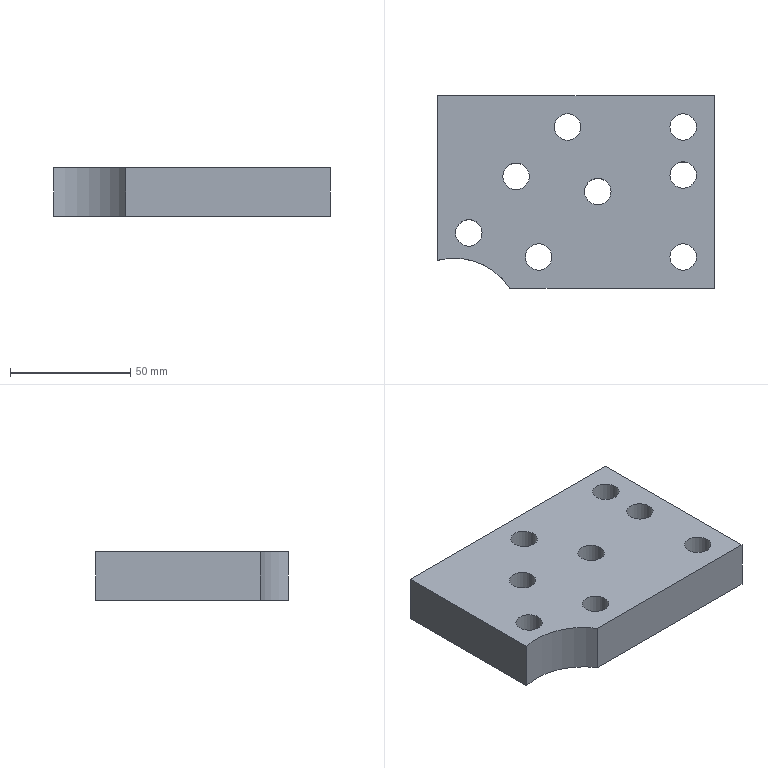Part | STEP file | 117_id2854_x_t | 1 solid | 15 faces | box 115 x 80 x 20 mm | volume 163028 mm3 | cylinder 9 | plane 6 | commonest cylinder face diameters 11 x8 55 x1
STEP:
#1=CARTESIAN_POINT('',(0.,0.,0.));
#2=DIRECTION('',(0.,0.,1.));
#3=DIRECTION('',(1.,0.,0.));
#4=AXIS2_PLACEMENT_3D('',#1,#2,#3);
#5=CARTESIAN_POINT('',(1208.57,-125.851,105.));
#6=VERTEX_POINT('',#5);
#7=CARTESIAN_POINT('',(1203.07,-125.851,105.));
#8=DIRECTION('',(0.,0.,-1.));
#9=DIRECTION('',(1.,0.,0.));
#10=AXIS2_PLACEMENT_3D('',#7,#8,#9);
#11=CIRCLE('',#10,5.5);
#12=CARTESIAN_POINT('',(1128.,-115.,105.));
#13=DIRECTION('',(0.,0.,1.));
#14=DIRECTION('',(-1.,0.,0.));
#15=AXIS2_PLACEMENT_3D('',#12,#13,#14);
#16=PLANE('',#15);
#17=CARTESIAN_POINT('',(-80.57,10.851));
#18=CARTESIAN_POINT('',(-80.57,20.377));
#19=CARTESIAN_POINT('',(-72.32,15.614));
#20=CARTESIAN_POINT('',(-64.07,10.851));
#21=CARTESIAN_POINT('',(-72.32,6.087));
#22=CARTESIAN_POINT('',(-80.57,1.324));
#23=CARTESIAN_POINT('',(-80.57,10.851));
#24=(BOUNDED_CURVE()B_SPLINE_CURVE(2,(#17,#18,#19,#20,#21,#22,#23),.UNSPECIFIED.,.T.,.F.)B_SPLINE_CURVE_WITH_KNOTS((1,2,2,2,2,1),(-2.094,0.,2.094,4.189,6.283,8.378),.UNSPECIFIED.)CURVE()GEOMETRIC_REPRESENTATION_ITEM()RATIONAL_B_SPLINE_CURVE((1.,0.5,1.,0.5,1.,0.5,1.))REPRESENTATION_ITEM(''));
#25=(GEOMETRIC_REPRESENTATION_CONTEXT(2)PARAMETRIC_REPRESENTATION_CONTEXT()REPRESENTATION_CONTEXT('',''));
#26=DEFINITIONAL_REPRESENTATION('',(#24),#25);
#27=PCURVE('',#16,#26);
#28=CARTESIAN_POINT('',(1203.07,-125.851,137.));
#29=DIRECTION('',(0.,0.,-1.));
#30=DIRECTION('',(1.,0.,0.));
#31=AXIS2_PLACEMENT_3D('',#28,#29,#30);
#32=CYLINDRICAL_SURFACE('',#31,5.5);
#33=CARTESIAN_POINT('',(0.,32.));
#34=DIRECTION('',(1.,0.));
#35=VECTOR('',#34,1.);
#36=LINE('',#33,#35);
#37=(GEOMETRIC_REPRESENTATION_CONTEXT(2)PARAMETRIC_REPRESENTATION_CONTEXT()REPRESENTATION_CONTEXT('',''));
#38=DEFINITIONAL_REPRESENTATION('',(#36),#37);
#39=PCURVE('',#32,#38);
#40=SURFACE_CURVE('',#11,(#27,#39),.PCURVE_S1.);
#41=EDGE_CURVE('',#6,#6,#40,.T.);
#42=ORIENTED_EDGE('',*,*,#41,.T.);
#43=EDGE_LOOP('',(#42));
#44=FACE_BOUND('',#43,.T.);
#45=CARTESIAN_POINT('',(1244.,-153.,105.));
#46=VERTEX_POINT('',#45);
#47=CARTESIAN_POINT('',(1233.,-153.,105.));
#48=VERTEX_POINT('',#47);
#49=CARTESIAN_POINT('',(1238.5,-153.,105.));
#50=DIRECTION('',(0.,0.,1.));
#51=DIRECTION('',(1.,0.,0.));
#52=AXIS2_PLACEMENT_3D('',#49,#50,#51);
#53=CIRCLE('',#52,5.5);
#54=CARTESIAN_POINT('',(-110.5,38.));
#55=DIRECTION('',(-1.,0.));
#56=AXIS2_PLACEMENT_2D('',#54,#55);
#57=CIRCLE('',#56,5.5);
#58=(GEOMETRIC_REPRESENTATION_CONTEXT(2)PARAMETRIC_REPRESENTATION_CONTEXT()REPRESENTATION_CONTEXT('',''));
#59=DEFINITIONAL_REPRESENTATION('',(#57),#58);
#60=PCURVE('',#16,#59);
#61=CARTESIAN_POINT('',(1238.5,-153.,90.));
#62=DIRECTION('',(0.,0.,1.));
#63=DIRECTION('',(-1.,0.,0.));
#64=AXIS2_PLACEMENT_3D('',#61,#62,#63);
#65=CYLINDRICAL_SURFACE('',#64,5.5);
#66=CARTESIAN_POINT('',(3.142,15.));
#67=DIRECTION('',(1.,0.));
#68=VECTOR('',#67,1.);
#69=LINE('',#66,#68);
#70=(GEOMETRIC_REPRESENTATION_CONTEXT(2)PARAMETRIC_REPRESENTATION_CONTEXT()REPRESENTATION_CONTEXT('',''));
#71=DEFINITIONAL_REPRESENTATION('',(#69),#70);
#72=PCURVE('',#65,#71);
#73=SURFACE_CURVE('',#53,(#60,#72),.PCURVE_S1.);
#74=EDGE_CURVE('',#46,#48,#73,.T.);
#75=ORIENTED_EDGE('',*,*,#74,.F.);
#76=CARTESIAN_POINT('',(1238.5,-153.,105.));
#77=DIRECTION('',(0.,0.,1.));
#78=DIRECTION('',(1.,0.,0.));
#79=AXIS2_PLACEMENT_3D('',#76,#77,#78);
#80=CIRCLE('',#79,5.5);
#81=CARTESIAN_POINT('',(-110.5,38.));
#82=DIRECTION('',(-1.,0.));
#83=AXIS2_PLACEMENT_2D('',#81,#82);
#84=CIRCLE('',#83,5.5);
#85=(GEOMETRIC_REPRESENTATION_CONTEXT(2)PARAMETRIC_REPRESENTATION_CONTEXT()REPRESENTATION_CONTEXT('',''));
#86=DEFINITIONAL_REPRESENTATION('',(#84),#85);
#87=PCURVE('',#16,#86);
#88=CARTESIAN_POINT('',(-3.142,15.));
#89=DIRECTION('',(1.,0.));
#90=VECTOR('',#89,1.);
#91=LINE('',#88,#90);
#92=(GEOMETRIC_REPRESENTATION_CONTEXT(2)PARAMETRIC_REPRESENTATION_CONTEXT()REPRESENTATION_CONTEXT('',''));
#93=DEFINITIONAL_REPRESENTATION('',(#91),#92);
#94=PCURVE('',#65,#93);
#95=SURFACE_CURVE('',#80,(#87,#94),.PCURVE_S1.);
#96=EDGE_CURVE('',#48,#46,#95,.T.);
#97=ORIENTED_EDGE('',*,*,#96,.F.);
#98=EDGE_LOOP('',(#75,#97));
#99=FACE_BOUND('',#98,.T.);
#100=CARTESIAN_POINT('',(1244.,-99.,105.));
#101=VERTEX_POINT('',#100);
#102=CARTESIAN_POINT('',(1233.,-99.,105.));
#103=VERTEX_POINT('',#102);
#104=CARTESIAN_POINT('',(1238.5,-99.,105.));
#105=DIRECTION('',(0.,0.,1.));
#106=DIRECTION('',(1.,0.,0.));
#107=AXIS2_PLACEMENT_3D('',#104,#105,#106);
#108=CIRCLE('',#107,5.5);
#109=CARTESIAN_POINT('',(-110.5,-16.));
#110=DIRECTION('',(-1.,0.));
#111=AXIS2_PLACEMENT_2D('',#109,#110);
#112=CIRCLE('',#111,5.5);
#113=(GEOMETRIC_REPRESENTATION_CONTEXT(2)PARAMETRIC_REPRESENTATION_CONTEXT()REPRESENTATION_CONTEXT('',''));
#114=DEFINITIONAL_REPRESENTATION('',(#112),#113);
#115=PCURVE('',#16,#114);
#116=CARTESIAN_POINT('',(1238.5,-99.,90.));
#117=DIRECTION('',(0.,0.,1.));
#118=DIRECTION('',(-1.,0.,0.));
#119=AXIS2_PLACEMENT_3D('',#116,#117,#118);
#120=CYLINDRICAL_SURFACE('',#119,5.5);
#121=CARTESIAN_POINT('',(3.142,15.));
#122=DIRECTION('',(1.,0.));
#123=VECTOR('',#122,1.);
#124=LINE('',#121,#123);
#125=(GEOMETRIC_REPRESENTATION_CONTEXT(2)PARAMETRIC_REPRESENTATION_CONTEXT()REPRESENTATION_CONTEXT('',''));
#126=DEFINITIONAL_REPRESENTATION('',(#124),#125);
#127=PCURVE('',#120,#126);
#128=SURFACE_CURVE('',#108,(#115,#127),.PCURVE_S1.);
#129=EDGE_CURVE('',#101,#103,#128,.T.);
#130=ORIENTED_EDGE('',*,*,#129,.F.);
#131=CARTESIAN_POINT('',(1238.5,-99.,105.));
#132=DIRECTION('',(0.,0.,1.));
#133=DIRECTION('',(1.,0.,0.));
#134=AXIS2_PLACEMENT_3D('',#131,#132,#133);
#135=CIRCLE('',#134,5.5);
#136=CARTESIAN_POINT('',(-110.5,-16.));
#137=DIRECTION('',(-1.,0.));
#138=AXIS2_PLACEMENT_2D('',#136,#137);
#139=CIRCLE('',#138,5.5);
#140=(GEOMETRIC_REPRESENTATION_CONTEXT(2)PARAMETRIC_REPRESENTATION_CONTEXT()REPRESENTATION_CONTEXT('',''));
#141=DEFINITIONAL_REPRESENTATION('',(#139),#140);
#142=PCURVE('',#16,#141);
#143=CARTESIAN_POINT('',(-3.142,15.));
#144=DIRECTION('',(1.,0.));
#145=VECTOR('',#144,1.);
#146=LINE('',#143,#145);
#147=(GEOMETRIC_REPRESENTATION_CONTEXT(2)PARAMETRIC_REPRESENTATION_CONTEXT()REPRESENTATION_CONTEXT('',''));
#148=DEFINITIONAL_REPRESENTATION('',(#146),#147);
#149=PCURVE('',#120,#148);
#150=SURFACE_CURVE('',#135,(#142,#149),.PCURVE_S1.);
#151=EDGE_CURVE('',#103,#101,#150,.T.);
#152=ORIENTED_EDGE('',*,*,#151,.F.);
#153=EDGE_LOOP('',(#130,#152));
#154=FACE_BOUND('',#153,.T.);
#155=CARTESIAN_POINT('',(1244.,-119.,105.));
#156=VERTEX_POINT('',#155);
#157=CARTESIAN_POINT('',(1238.5,-119.,105.));
#158=DIRECTION('',(0.,0.,1.));
#159=DIRECTION('',(1.,0.,0.));
#160=AXIS2_PLACEMENT_3D('',#157,#158,#159);
#161=CIRCLE('',#160,5.5);
#162=CARTESIAN_POINT('',(-110.5,4.));
#163=DIRECTION('',(-1.,0.));
#164=AXIS2_PLACEMENT_2D('',#162,#163);
#165=CIRCLE('',#164,5.5);
#166=(GEOMETRIC_REPRESENTATION_CONTEXT(2)PARAMETRIC_REPRESENTATION_CONTEXT()REPRESENTATION_CONTEXT('',''));
#167=DEFINITIONAL_REPRESENTATION('',(#165),#166);
#168=PCURVE('',#16,#167);
#169=CARTESIAN_POINT('',(1238.5,-119.,90.));
#170=DIRECTION('',(0.,0.,1.));
#171=DIRECTION('',(0.,-1.,0.));
#172=AXIS2_PLACEMENT_3D('',#169,#170,#171);
#173=CYLINDRICAL_SURFACE('',#172,5.5);
#174=CARTESIAN_POINT('',(1.571,15.));
#175=DIRECTION('',(1.,0.));
#176=VECTOR('',#175,1.);
#177=LINE('',#174,#176);
#178=(GEOMETRIC_REPRESENTATION_CONTEXT(2)PARAMETRIC_REPRESENTATION_CONTEXT()REPRESENTATION_CONTEXT('',''));
#179=DEFINITIONAL_REPRESENTATION('',(#177),#178);
#180=PCURVE('',#173,#179);
#181=SURFACE_CURVE('',#161,(#168,#180),.PCURVE_S1.);
#182=EDGE_CURVE('',#156,#156,#181,.T.);
#183=ORIENTED_EDGE('',*,*,#182,.F.);
#184=EDGE_LOOP('',(#183));
#185=FACE_BOUND('',#184,.T.);
#186=CARTESIAN_POINT('',(1174.607,-119.53,105.));
#187=VERTEX_POINT('',#186);
#188=CARTESIAN_POINT('',(1169.107,-119.53,105.));
#189=DIRECTION('',(0.,0.,1.));
#190=DIRECTION('',(1.,0.,0.));
#191=AXIS2_PLACEMENT_3D('',#188,#189,#190);
#192=CIRCLE('',#191,5.5);
#193=CARTESIAN_POINT('',(-41.107,4.53));
#194=DIRECTION('',(-1.,0.));
#195=AXIS2_PLACEMENT_2D('',#193,#194);
#196=CIRCLE('',#195,5.5);
#197=(GEOMETRIC_REPRESENTATION_CONTEXT(2)PARAMETRIC_REPRESENTATION_CONTEXT()REPRESENTATION_CONTEXT('',''));
#198=DEFINITIONAL_REPRESENTATION('',(#196),#197);
#199=PCURVE('',#16,#198);
#200=CARTESIAN_POINT('',(1169.107,-119.53,137.));
#201=DIRECTION('',(0.,0.,-1.));
#202=DIRECTION('',(1.,0.,0.));
#203=AXIS2_PLACEMENT_3D('',#200,#201,#202);
#204=CYLINDRICAL_SURFACE('',#203,5.5);
#205=CARTESIAN_POINT('',(6.283,32.));
#206=DIRECTION('',(-1.,0.));
#207=VECTOR('',#206,1.);
#208=LINE('',#205,#207);
#209=(GEOMETRIC_REPRESENTATION_CONTEXT(2)PARAMETRIC_REPRESENTATION_CONTEXT()REPRESENTATION_CONTEXT('',''));
#210=DEFINITIONAL_REPRESENTATION('',(#208),#209);
#211=PCURVE('',#204,#210);
#212=SURFACE_CURVE('',#192,(#199,#211),.PCURVE_S1.);
#213=EDGE_CURVE('',#187,#187,#212,.T.);
#214=ORIENTED_EDGE('',*,*,#213,.F.);
#215=EDGE_LOOP('',(#214));
#216=FACE_BOUND('',#215,.T.);
#217=CARTESIAN_POINT('',(1136.5,-86.,105.));
#218=VERTEX_POINT('',#217);
#219=CARTESIAN_POINT('',(1136.5,-154.406,105.));
#220=VERTEX_POINT('',#219);
#221=CARTESIAN_POINT('',(1136.5,-126.,105.));
#222=DIRECTION('',(0.,-1.,0.));
#223=VECTOR('',#222,1.);
#224=LINE('',#221,#223);
#225=CARTESIAN_POINT('',(-8.5,11.));
#226=DIRECTION('',(0.,1.));
#227=VECTOR('',#226,1.);
#228=LINE('',#225,#227);
#229=(GEOMETRIC_REPRESENTATION_CONTEXT(2)PARAMETRIC_REPRESENTATION_CONTEXT()REPRESENTATION_CONTEXT('',''));
#230=DEFINITIONAL_REPRESENTATION('',(#228),#229);
#231=PCURVE('',#16,#230);
#232=CARTESIAN_POINT('',(1136.5,-126.,75.));
#233=DIRECTION('',(1.,0.,0.));
#234=DIRECTION('',(0.,0.,1.));
#235=AXIS2_PLACEMENT_3D('',#232,#233,#234);
#236=PLANE('',#235);
#237=CARTESIAN_POINT('',(30.,0.));
#238=DIRECTION('',(0.,1.));
#239=VECTOR('',#238,1.);
#240=LINE('',#237,#239);
#241=(GEOMETRIC_REPRESENTATION_CONTEXT(2)PARAMETRIC_REPRESENTATION_CONTEXT()REPRESENTATION_CONTEXT('',''));
#242=DEFINITIONAL_REPRESENTATION('',(#240),#241);
#243=PCURVE('',#236,#242);
#244=SURFACE_CURVE('',#224,(#231,#243),.PCURVE_S1.);
#245=EDGE_CURVE('',#218,#220,#244,.T.);
#246=ORIENTED_EDGE('',*,*,#245,.T.);
#247=CARTESIAN_POINT('',(1166.549,-166.,105.));
#248=VERTEX_POINT('',#247);
#249=CARTESIAN_POINT('',(1143.5,-181.,105.));
#250=DIRECTION('',(0.,0.,1.));
#251=DIRECTION('',(1.,0.,0.));
#252=AXIS2_PLACEMENT_3D('',#249,#250,#251);
#253=CIRCLE('',#252,27.5);
#254=CARTESIAN_POINT('',(-15.5,66.));
#255=DIRECTION('',(-1.,0.));
#256=AXIS2_PLACEMENT_2D('',#254,#255);
#257=CIRCLE('',#256,27.5);
#258=(GEOMETRIC_REPRESENTATION_CONTEXT(2)PARAMETRIC_REPRESENTATION_CONTEXT()REPRESENTATION_CONTEXT('',''));
#259=DEFINITIONAL_REPRESENTATION('',(#257),#258);
#260=PCURVE('',#16,#259);
#261=CARTESIAN_POINT('',(1143.5,-181.,400.));
#262=DIRECTION('',(0.,0.,-1.));
#263=DIRECTION('',(1.,0.,0.));
#264=AXIS2_PLACEMENT_3D('',#261,#262,#263);
#265=CYLINDRICAL_SURFACE('',#264,27.5);
#266=CARTESIAN_POINT('',(6.283,295.));
#267=DIRECTION('',(-1.,0.));
#268=VECTOR('',#267,1.);
#269=LINE('',#266,#268);
#270=(GEOMETRIC_REPRESENTATION_CONTEXT(2)PARAMETRIC_REPRESENTATION_CONTEXT()REPRESENTATION_CONTEXT('',''));
#271=DEFINITIONAL_REPRESENTATION('',(#269),#270);
#272=PCURVE('',#265,#271);
#273=SURFACE_CURVE('',#253,(#260,#272),.PCURVE_S1.);
#274=EDGE_CURVE('',#248,#220,#273,.T.);
#275=ORIENTED_EDGE('',*,*,#274,.F.);
#276=CARTESIAN_POINT('',(1251.5,-166.,105.));
#277=VERTEX_POINT('',#276);
#278=CARTESIAN_POINT('',(1128.,-166.,105.));
#279=DIRECTION('',(1.,0.,0.));
#280=VECTOR('',#279,1.);
#281=LINE('',#278,#280);
#282=CARTESIAN_POINT('',(0.,51.));
#283=DIRECTION('',(-1.,0.));
#284=VECTOR('',#283,1.);
#285=LINE('',#282,#284);
#286=(GEOMETRIC_REPRESENTATION_CONTEXT(2)PARAMETRIC_REPRESENTATION_CONTEXT()REPRESENTATION_CONTEXT('',''));
#287=DEFINITIONAL_REPRESENTATION('',(#285),#286);
#288=PCURVE('',#16,#287);
#289=CARTESIAN_POINT('',(1128.,-166.,90.));
#290=DIRECTION('',(0.,-1.,0.));
#291=DIRECTION('',(0.,0.,1.));
#292=AXIS2_PLACEMENT_3D('',#289,#290,#291);
#293=PLANE('',#292);
#294=CARTESIAN_POINT('',(15.,0.));
#295=DIRECTION('',(0.,-1.));
#296=VECTOR('',#295,1.);
#297=LINE('',#294,#296);
#298=(GEOMETRIC_REPRESENTATION_CONTEXT(2)PARAMETRIC_REPRESENTATION_CONTEXT()REPRESENTATION_CONTEXT('',''));
#299=DEFINITIONAL_REPRESENTATION('',(#297),#298);
#300=PCURVE('',#293,#299);
#301=SURFACE_CURVE('',#281,(#288,#300),.PCURVE_S1.);
#302=EDGE_CURVE('',#248,#277,#301,.T.);
#303=ORIENTED_EDGE('',*,*,#302,.T.);
#304=CARTESIAN_POINT('',(1251.5,-86.,105.));
#305=VERTEX_POINT('',#304);
#306=CARTESIAN_POINT('',(1251.5,-115.,105.));
#307=DIRECTION('',(0.,1.,0.));
#308=VECTOR('',#307,1.);
#309=LINE('',#306,#308);
#310=CARTESIAN_POINT('',(-123.5,0.));
#311=DIRECTION('',(0.,-1.));
#312=VECTOR('',#311,1.);
#313=LINE('',#310,#312);
#314=(GEOMETRIC_REPRESENTATION_CONTEXT(2)PARAMETRIC_REPRESENTATION_CONTEXT()REPRESENTATION_CONTEXT('',''));
#315=DEFINITIONAL_REPRESENTATION('',(#313),#314);
#316=PCURVE('',#16,#315);
#317=CARTESIAN_POINT('',(1251.5,-115.,90.));
#318=DIRECTION('',(1.,0.,0.));
#319=DIRECTION('',(0.,0.,1.));
#320=AXIS2_PLACEMENT_3D('',#317,#318,#319);
#321=PLANE('',#320);
#322=CARTESIAN_POINT('',(15.,0.));
#323=DIRECTION('',(0.,-1.));
#324=VECTOR('',#323,1.);
#325=LINE('',#322,#324);
#326=(GEOMETRIC_REPRESENTATION_CONTEXT(2)PARAMETRIC_REPRESENTATION_CONTEXT()REPRESENTATION_CONTEXT('',''));
#327=DEFINITIONAL_REPRESENTATION('',(#325),#326);
#328=PCURVE('',#321,#327);
#329=SURFACE_CURVE('',#309,(#316,#328),.PCURVE_S1.);
#330=EDGE_CURVE('',#277,#305,#329,.T.);
#331=ORIENTED_EDGE('',*,*,#330,.T.);
#332=CARTESIAN_POINT('',(1128.,-86.,105.));
#333=DIRECTION('',(-1.,0.,0.));
#334=VECTOR('',#333,1.);
#335=LINE('',#332,#334);
#336=CARTESIAN_POINT('',(0.,-29.));
#337=DIRECTION('',(1.,0.));
#338=VECTOR('',#337,1.);
#339=LINE('',#336,#338);
#340=(GEOMETRIC_REPRESENTATION_CONTEXT(2)PARAMETRIC_REPRESENTATION_CONTEXT()REPRESENTATION_CONTEXT('',''));
#341=DEFINITIONAL_REPRESENTATION('',(#339),#340);
#342=PCURVE('',#16,#341);
#343=CARTESIAN_POINT('',(1128.,-86.,90.));
#344=DIRECTION('',(0.,1.,0.));
#345=DIRECTION('',(0.,0.,-1.));
#346=AXIS2_PLACEMENT_3D('',#343,#344,#345);
#347=PLANE('',#346);
#348=CARTESIAN_POINT('',(-15.,0.));
#349=DIRECTION('',(0.,1.));
#350=VECTOR('',#349,1.);
#351=LINE('',#348,#350);
#352=(GEOMETRIC_REPRESENTATION_CONTEXT(2)PARAMETRIC_REPRESENTATION_CONTEXT()REPRESENTATION_CONTEXT('',''));
#353=DEFINITIONAL_REPRESENTATION('',(#351),#352);
#354=PCURVE('',#347,#353);
#355=SURFACE_CURVE('',#335,(#342,#354),.PCURVE_S1.);
#356=EDGE_CURVE('',#305,#218,#355,.T.);
#357=ORIENTED_EDGE('',*,*,#356,.T.);
#358=EDGE_LOOP('',(#246,#275,#303,#331,#357));
#359=FACE_BOUND('',#358,.T.);
#360=CARTESIAN_POINT('',(1184.,-153.,105.));
#361=VERTEX_POINT('',#360);
#362=CARTESIAN_POINT('',(1178.5,-153.,105.));
#363=DIRECTION('',(0.,0.,1.));
#364=DIRECTION('',(1.,0.,0.));
#365=AXIS2_PLACEMENT_3D('',#362,#363,#364);
#366=CIRCLE('',#365,5.5);
#367=CARTESIAN_POINT('',(-50.5,38.));
#368=DIRECTION('',(-1.,0.));
#369=AXIS2_PLACEMENT_2D('',#367,#368);
#370=CIRCLE('',#369,5.5);
#371=(GEOMETRIC_REPRESENTATION_CONTEXT(2)PARAMETRIC_REPRESENTATION_CONTEXT()REPRESENTATION_CONTEXT('',''));
#372=DEFINITIONAL_REPRESENTATION('',(#370),#371);
#373=PCURVE('',#16,#372);
#374=CARTESIAN_POINT('',(1178.5,-153.,280.));
#375=DIRECTION('',(0.,0.,-1.));
#376=DIRECTION('',(1.,0.,0.));
#377=AXIS2_PLACEMENT_3D('',#374,#375,#376);
#378=CYLINDRICAL_SURFACE('',#377,5.5);
#379=CARTESIAN_POINT('',(6.283,175.));
#380=DIRECTION('',(-1.,0.));
#381=VECTOR('',#380,1.);
#382=LINE('',#379,#381);
#383=(GEOMETRIC_REPRESENTATION_CONTEXT(2)PARAMETRIC_REPRESENTATION_CONTEXT()REPRESENTATION_CONTEXT('',''));
#384=DEFINITIONAL_REPRESENTATION('',(#382),#383);
#385=PCURVE('',#378,#384);
#386=SURFACE_CURVE('',#366,(#373,#385),.PCURVE_S1.);
#387=EDGE_CURVE('',#361,#361,#386,.T.);
#388=ORIENTED_EDGE('',*,*,#387,.F.);
#389=EDGE_LOOP('',(#388));
#390=FACE_BOUND('',#389,.T.);
#391=CARTESIAN_POINT('',(1196.,-99.,105.));
#392=VERTEX_POINT('',#391);
#393=CARTESIAN_POINT('',(1190.5,-99.,105.));
#394=DIRECTION('',(0.,0.,1.));
#395=DIRECTION('',(1.,0.,0.));
#396=AXIS2_PLACEMENT_3D('',#393,#394,#395);
#397=CIRCLE('',#396,5.5);
#398=CARTESIAN_POINT('',(-62.5,-16.));
#399=DIRECTION('',(-1.,0.));
#400=AXIS2_PLACEMENT_2D('',#398,#399);
#401=CIRCLE('',#400,5.5);
#402=(GEOMETRIC_REPRESENTATION_CONTEXT(2)PARAMETRIC_REPRESENTATION_CONTEXT()REPRESENTATION_CONTEXT('',''));
#403=DEFINITIONAL_REPRESENTATION('',(#401),#402);
#404=PCURVE('',#16,#403);
#405=CARTESIAN_POINT('',(1190.5,-99.,280.));
#406=DIRECTION('',(0.,0.,-1.));
#407=DIRECTION('',(1.,0.,0.));
#408=AXIS2_PLACEMENT_3D('',#405,#406,#407);
#409=CYLINDRICAL_SURFACE('',#408,5.5);
#410=CARTESIAN_POINT('',(6.283,175.));
#411=DIRECTION('',(-1.,0.));
#412=VECTOR('',#411,1.);
#413=LINE('',#410,#412);
#414=(GEOMETRIC_REPRESENTATION_CONTEXT(2)PARAMETRIC_REPRESENTATION_CONTEXT()REPRESENTATION_CONTEXT('',''));
#415=DEFINITIONAL_REPRESENTATION('',(#413),#414);
#416=PCURVE('',#409,#415);
#417=SURFACE_CURVE('',#397,(#404,#416),.PCURVE_S1.);
#418=EDGE_CURVE('',#392,#392,#417,.T.);
#419=ORIENTED_EDGE('',*,*,#418,.F.);
#420=EDGE_LOOP('',(#419));
#421=FACE_BOUND('',#420,.T.);
#422=CARTESIAN_POINT('',(1155.,-143.,105.));
#423=VERTEX_POINT('',#422);
#424=CARTESIAN_POINT('',(1149.5,-143.,105.));
#425=DIRECTION('',(0.,0.,-1.));
#426=DIRECTION('',(1.,0.,0.));
#427=AXIS2_PLACEMENT_3D('',#424,#425,#426);
#428=CIRCLE('',#427,5.5);
#429=CARTESIAN_POINT('',(-27.,28.));
#430=CARTESIAN_POINT('',(-27.,37.526));
#431=CARTESIAN_POINT('',(-18.75,32.763));
#432=CARTESIAN_POINT('',(-10.5,28.));
#433=CARTESIAN_POINT('',(-18.75,23.237));
#434=CARTESIAN_POINT('',(-27.,18.474));
#435=CARTESIAN_POINT('',(-27.,28.));
#436=(BOUNDED_CURVE()B_SPLINE_CURVE(2,(#429,#430,#431,#432,#433,#434,#435),.UNSPECIFIED.,.T.,.F.)B_SPLINE_CURVE_WITH_KNOTS((1,2,2,2,2,1),(-2.094,0.,2.094,4.189,6.283,8.378),.UNSPECIFIED.)CURVE()GEOMETRIC_REPRESENTATION_ITEM()RATIONAL_B_SPLINE_CURVE((1.,0.5,1.,0.5,1.,0.5,1.))REPRESENTATION_ITEM(''));
#437=(GEOMETRIC_REPRESENTATION_CONTEXT(2)PARAMETRIC_REPRESENTATION_CONTEXT()REPRESENTATION_CONTEXT('',''));
#438=DEFINITIONAL_REPRESENTATION('',(#436),#437);
#439=PCURVE('',#16,#438);
#440=CARTESIAN_POINT('',(1149.5,-143.,265.));
#441=DIRECTION('',(0.,0.,-1.));
#442=DIRECTION('',(1.,0.,0.));
#443=AXIS2_PLACEMENT_3D('',#440,#441,#442);
#444=CYLINDRICAL_SURFACE('',#443,5.5);
#445=CARTESIAN_POINT('',(0.,160.));
#446=DIRECTION('',(1.,0.));
#447=VECTOR('',#446,1.);
#448=LINE('',#445,#447);
#449=(GEOMETRIC_REPRESENTATION_CONTEXT(2)PARAMETRIC_REPRESENTATION_CONTEXT()REPRESENTATION_CONTEXT('',''));
#450=DEFINITIONAL_REPRESENTATION('',(#448),#449);
#451=PCURVE('',#444,#450);
#452=SURFACE_CURVE('',#428,(#439,#451),.PCURVE_S1.);
#453=EDGE_CURVE('',#423,#423,#452,.T.);
#454=ORIENTED_EDGE('',*,*,#453,.T.);
#455=EDGE_LOOP('',(#454));
#456=FACE_BOUND('',#455,.T.);
#457=ADVANCED_FACE('',(#44,#99,#154,#185,#216,#359,#390,#421,#456),#16,.T.);
#458=CARTESIAN_POINT('',(1197.57,-125.851,85.));
#459=VERTEX_POINT('',#458);
#460=CARTESIAN_POINT('',(1208.57,-125.851,85.));
#461=VERTEX_POINT('',#460);
#462=CARTESIAN_POINT('',(1203.07,-125.851,85.));
#463=DIRECTION('',(0.,0.,1.));
#464=DIRECTION('',(-1.,0.,0.));
#465=AXIS2_PLACEMENT_3D('',#462,#463,#464);
#466=CIRCLE('',#465,5.5);
#467=CARTESIAN_POINT('',(1128.,-115.,85.));
#468=DIRECTION('',(0.,0.,-1.));
#469=DIRECTION('',(1.,0.,0.));
#470=AXIS2_PLACEMENT_3D('',#467,#468,#469);
#471=PLANE('',#470);
#472=CARTESIAN_POINT('',(69.57,10.851));
#473=CARTESIAN_POINT('',(69.57,20.377));
#474=CARTESIAN_POINT('',(77.82,15.614));
#475=CARTESIAN_POINT('',(86.07,10.851));
#476=CARTESIAN_POINT('',(77.82,6.087));
#477=CARTESIAN_POINT('',(69.57,1.324));
#478=CARTESIAN_POINT('',(69.57,10.851));
#479=(BOUNDED_CURVE()B_SPLINE_CURVE(2,(#472,#473,#474,#475,#476,#477,#478),.UNSPECIFIED.,.T.,.F.)B_SPLINE_CURVE_WITH_KNOTS((1,2,2,2,2,1),(-2.094,0.,2.094,4.189,6.283,8.378),.UNSPECIFIED.)CURVE()GEOMETRIC_REPRESENTATION_ITEM()RATIONAL_B_SPLINE_CURVE((1.,0.5,1.,0.5,1.,0.5,1.))REPRESENTATION_ITEM(''));
#480=(GEOMETRIC_REPRESENTATION_CONTEXT(2)PARAMETRIC_REPRESENTATION_CONTEXT()REPRESENTATION_CONTEXT('',''));
#481=DEFINITIONAL_REPRESENTATION('',(#479),#480);
#482=PCURVE('',#471,#481);
#483=CARTESIAN_POINT('',(3.142,52.));
#484=DIRECTION('',(-1.,0.));
#485=VECTOR('',#484,1.);
#486=LINE('',#483,#485);
#487=(GEOMETRIC_REPRESENTATION_CONTEXT(2)PARAMETRIC_REPRESENTATION_CONTEXT()REPRESENTATION_CONTEXT('',''));
#488=DEFINITIONAL_REPRESENTATION('',(#486),#487);
#489=PCURVE('',#32,#488);
#490=SURFACE_CURVE('',#466,(#482,#489),.PCURVE_S1.);
#491=EDGE_CURVE('',#459,#461,#490,.T.);
#492=ORIENTED_EDGE('',*,*,#491,.T.);
#493=CARTESIAN_POINT('',(1203.07,-125.851,85.));
#494=DIRECTION('',(0.,0.,1.));
#495=DIRECTION('',(-1.,0.,0.));
#496=AXIS2_PLACEMENT_3D('',#493,#494,#495);
#497=CIRCLE('',#496,5.5);
#498=CARTESIAN_POINT('',(69.57,10.851));
#499=CARTESIAN_POINT('',(69.57,20.377));
#500=CARTESIAN_POINT('',(77.82,15.614));
#501=CARTESIAN_POINT('',(86.07,10.851));
#502=CARTESIAN_POINT('',(77.82,6.087));
#503=CARTESIAN_POINT('',(69.57,1.324));
#504=CARTESIAN_POINT('',(69.57,10.851));
#505=(BOUNDED_CURVE()B_SPLINE_CURVE(2,(#498,#499,#500,#501,#502,#503,#504),.UNSPECIFIED.,.T.,.F.)B_SPLINE_CURVE_WITH_KNOTS((1,2,2,2,2,1),(-2.094,0.,2.094,4.189,6.283,8.378),.UNSPECIFIED.)CURVE()GEOMETRIC_REPRESENTATION_ITEM()RATIONAL_B_SPLINE_CURVE((1.,0.5,1.,0.5,1.,0.5,1.))REPRESENTATION_ITEM(''));
#506=(GEOMETRIC_REPRESENTATION_CONTEXT(2)PARAMETRIC_REPRESENTATION_CONTEXT()REPRESENTATION_CONTEXT('',''));
#507=DEFINITIONAL_REPRESENTATION('',(#505),#506);
#508=PCURVE('',#471,#507);
#509=CARTESIAN_POINT('',(9.425,52.));
#510=DIRECTION('',(-1.,0.));
#511=VECTOR('',#510,1.);
#512=LINE('',#509,#511);
#513=(GEOMETRIC_REPRESENTATION_CONTEXT(2)PARAMETRIC_REPRESENTATION_CONTEXT()REPRESENTATION_CONTEXT('',''));
#514=DEFINITIONAL_REPRESENTATION('',(#512),#513);
#515=PCURVE('',#32,#514);
#516=SURFACE_CURVE('',#497,(#508,#515),.PCURVE_S1.);
#517=EDGE_CURVE('',#461,#459,#516,.T.);
#518=ORIENTED_EDGE('',*,*,#517,.T.);
#519=EDGE_LOOP('',(#492,#518));
#520=FACE_BOUND('',#519,.T.);
#521=CARTESIAN_POINT('',(1233.,-99.,85.));
#522=VERTEX_POINT('',#521);
#523=CARTESIAN_POINT('',(1238.5,-99.,85.));
#524=DIRECTION('',(0.,0.,-1.));
#525=DIRECTION('',(-1.,0.,0.));
#526=AXIS2_PLACEMENT_3D('',#523,#524,#525);
#527=CIRCLE('',#526,5.5);
#528=CARTESIAN_POINT('',(110.5,-16.));
#529=DIRECTION('',(-1.,0.));
#530=AXIS2_PLACEMENT_2D('',#528,#529);
#531=CIRCLE('',#530,5.5);
#532=(GEOMETRIC_REPRESENTATION_CONTEXT(2)PARAMETRIC_REPRESENTATION_CONTEXT()REPRESENTATION_CONTEXT('',''));
#533=DEFINITIONAL_REPRESENTATION('',(#531),#532);
#534=PCURVE('',#471,#533);
#535=CARTESIAN_POINT('',(6.283,-5.));
#536=DIRECTION('',(-1.,0.));
#537=VECTOR('',#536,1.);
#538=LINE('',#535,#537);
#539=(GEOMETRIC_REPRESENTATION_CONTEXT(2)PARAMETRIC_REPRESENTATION_CONTEXT()REPRESENTATION_CONTEXT('',''));
#540=DEFINITIONAL_REPRESENTATION('',(#538),#539);
#541=PCURVE('',#120,#540);
#542=SURFACE_CURVE('',#527,(#534,#541),.PCURVE_S1.);
#543=EDGE_CURVE('',#522,#522,#542,.T.);
#544=ORIENTED_EDGE('',*,*,#543,.F.);
#545=EDGE_LOOP('',(#544));
#546=FACE_BOUND('',#545,.T.);
#547=CARTESIAN_POINT('',(1233.,-119.,85.));
#548=VERTEX_POINT('',#547);
#549=CARTESIAN_POINT('',(1244.,-119.,85.));
#550=VERTEX_POINT('',#549);
#551=CARTESIAN_POINT('',(1238.5,-119.,85.));
#552=DIRECTION('',(0.,0.,-1.));
#553=DIRECTION('',(-1.,0.,0.));
#554=AXIS2_PLACEMENT_3D('',#551,#552,#553);
#555=CIRCLE('',#554,5.5);
#556=CARTESIAN_POINT('',(110.5,4.));
#557=DIRECTION('',(-1.,0.));
#558=AXIS2_PLACEMENT_2D('',#556,#557);
#559=CIRCLE('',#558,5.5);
#560=(GEOMETRIC_REPRESENTATION_CONTEXT(2)PARAMETRIC_REPRESENTATION_CONTEXT()REPRESENTATION_CONTEXT('',''));
#561=DEFINITIONAL_REPRESENTATION('',(#559),#560);
#562=PCURVE('',#471,#561);
#563=CARTESIAN_POINT('',(4.712,-5.));
#564=DIRECTION('',(-1.,0.));
#565=VECTOR('',#564,1.);
#566=LINE('',#563,#565);
#567=(GEOMETRIC_REPRESENTATION_CONTEXT(2)PARAMETRIC_REPRESENTATION_CONTEXT()REPRESENTATION_CONTEXT('',''));
#568=DEFINITIONAL_REPRESENTATION('',(#566),#567);
#569=PCURVE('',#173,#568);
#570=SURFACE_CURVE('',#555,(#562,#569),.PCURVE_S1.);
#571=EDGE_CURVE('',#548,#550,#570,.T.);
#572=ORIENTED_EDGE('',*,*,#571,.F.);
#573=CARTESIAN_POINT('',(1238.5,-119.,85.));
#574=DIRECTION('',(0.,0.,-1.));
#575=DIRECTION('',(-1.,0.,0.));
#576=AXIS2_PLACEMENT_3D('',#573,#574,#575);
#577=CIRCLE('',#576,5.5);
#578=CARTESIAN_POINT('',(110.5,4.));
#579=DIRECTION('',(-1.,0.));
#580=AXIS2_PLACEMENT_2D('',#578,#579);
#581=CIRCLE('',#580,5.5);
#582=(GEOMETRIC_REPRESENTATION_CONTEXT(2)PARAMETRIC_REPRESENTATION_CONTEXT()REPRESENTATION_CONTEXT('',''));
#583=DEFINITIONAL_REPRESENTATION('',(#581),#582);
#584=PCURVE('',#471,#583);
#585=CARTESIAN_POINT('',(10.996,-5.));
#586=DIRECTION('',(-1.,0.));
#587=VECTOR('',#586,1.);
#588=LINE('',#585,#587);
#589=(GEOMETRIC_REPRESENTATION_CONTEXT(2)PARAMETRIC_REPRESENTATION_CONTEXT()REPRESENTATION_CONTEXT('',''));
#590=DEFINITIONAL_REPRESENTATION('',(#588),#589);
#591=PCURVE('',#173,#590);
#592=SURFACE_CURVE('',#577,(#584,#591),.PCURVE_S1.);
#593=EDGE_CURVE('',#550,#548,#592,.T.);
#594=ORIENTED_EDGE('',*,*,#593,.F.);
#595=EDGE_LOOP('',(#572,#594));
#596=FACE_BOUND('',#595,.T.);
#597=CARTESIAN_POINT('',(1233.,-153.,85.));
#598=VERTEX_POINT('',#597);
#599=CARTESIAN_POINT('',(1238.5,-153.,85.));
#600=DIRECTION('',(0.,0.,-1.));
#601=DIRECTION('',(-1.,0.,0.));
#602=AXIS2_PLACEMENT_3D('',#599,#600,#601);
#603=CIRCLE('',#602,5.5);
#604=CARTESIAN_POINT('',(110.5,38.));
#605=DIRECTION('',(-1.,0.));
#606=AXIS2_PLACEMENT_2D('',#604,#605);
#607=CIRCLE('',#606,5.5);
#608=(GEOMETRIC_REPRESENTATION_CONTEXT(2)PARAMETRIC_REPRESENTATION_CONTEXT()REPRESENTATION_CONTEXT('',''));
#609=DEFINITIONAL_REPRESENTATION('',(#607),#608);
#610=PCURVE('',#471,#609);
#611=CARTESIAN_POINT('',(6.283,-5.));
#612=DIRECTION('',(-1.,0.));
#613=VECTOR('',#612,1.);
#614=LINE('',#611,#613);
#615=(GEOMETRIC_REPRESENTATION_CONTEXT(2)PARAMETRIC_REPRESENTATION_CONTEXT()REPRESENTATION_CONTEXT('',''));
#616=DEFINITIONAL_REPRESENTATION('',(#614),#615);
#617=PCURVE('',#65,#616);
#618=SURFACE_CURVE('',#603,(#610,#617),.PCURVE_S1.);
#619=EDGE_CURVE('',#598,#598,#618,.T.);
#620=ORIENTED_EDGE('',*,*,#619,.F.);
#621=EDGE_LOOP('',(#620));
#622=FACE_BOUND('',#621,.T.);
#623=CARTESIAN_POINT('',(1163.607,-119.53,85.));
#624=VERTEX_POINT('',#623);
#625=CARTESIAN_POINT('',(1174.607,-119.53,85.));
#626=VERTEX_POINT('',#625);
#627=CARTESIAN_POINT('',(1169.107,-119.53,85.));
#628=DIRECTION('',(0.,0.,-1.));
#629=DIRECTION('',(-1.,0.,0.));
#630=AXIS2_PLACEMENT_3D('',#627,#628,#629);
#631=CIRCLE('',#630,5.5);
#632=CARTESIAN_POINT('',(41.107,4.53));
#633=DIRECTION('',(-1.,0.));
#634=AXIS2_PLACEMENT_2D('',#632,#633);
#635=CIRCLE('',#634,5.5);
#636=(GEOMETRIC_REPRESENTATION_CONTEXT(2)PARAMETRIC_REPRESENTATION_CONTEXT()REPRESENTATION_CONTEXT('',''));
#637=DEFINITIONAL_REPRESENTATION('',(#635),#636);
#638=PCURVE('',#471,#637);
#639=CARTESIAN_POINT('',(3.142,52.));
#640=DIRECTION('',(1.,0.));
#641=VECTOR('',#640,1.);
#642=LINE('',#639,#641);
#643=(GEOMETRIC_REPRESENTATION_CONTEXT(2)PARAMETRIC_REPRESENTATION_CONTEXT()REPRESENTATION_CONTEXT('',''));
#644=DEFINITIONAL_REPRESENTATION('',(#642),#643);
#645=PCURVE('',#204,#644);
#646=SURFACE_CURVE('',#631,(#638,#645),.PCURVE_S1.);
#647=EDGE_CURVE('',#624,#626,#646,.T.);
#648=ORIENTED_EDGE('',*,*,#647,.F.);
#649=CARTESIAN_POINT('',(1169.107,-119.53,85.));
#650=DIRECTION('',(0.,0.,-1.));
#651=DIRECTION('',(-1.,0.,0.));
#652=AXIS2_PLACEMENT_3D('',#649,#650,#651);
#653=CIRCLE('',#652,5.5);
#654=CARTESIAN_POINT('',(41.107,4.53));
#655=DIRECTION('',(-1.,0.));
#656=AXIS2_PLACEMENT_2D('',#654,#655);
#657=CIRCLE('',#656,5.5);
#658=(GEOMETRIC_REPRESENTATION_CONTEXT(2)PARAMETRIC_REPRESENTATION_CONTEXT()REPRESENTATION_CONTEXT('',''));
#659=DEFINITIONAL_REPRESENTATION('',(#657),#658);
#660=PCURVE('',#471,#659);
#661=CARTESIAN_POINT('',(-3.142,52.));
#662=DIRECTION('',(1.,0.));
#663=VECTOR('',#662,1.);
#664=LINE('',#661,#663);
#665=(GEOMETRIC_REPRESENTATION_CONTEXT(2)PARAMETRIC_REPRESENTATION_CONTEXT()REPRESENTATION_CONTEXT('',''));
#666=DEFINITIONAL_REPRESENTATION('',(#664),#665);
#667=PCURVE('',#204,#666);
#668=SURFACE_CURVE('',#653,(#660,#667),.PCURVE_S1.);
#669=EDGE_CURVE('',#626,#624,#668,.T.);
#670=ORIENTED_EDGE('',*,*,#669,.F.);
#671=EDGE_LOOP('',(#648,#670));
#672=FACE_BOUND('',#671,.T.);
#673=CARTESIAN_POINT('',(1136.5,-154.406,85.));
#674=VERTEX_POINT('',#673);
#675=CARTESIAN_POINT('',(1136.5,-86.,85.));
#676=VERTEX_POINT('',#675);
#677=CARTESIAN_POINT('',(1136.5,-126.,85.));
#678=DIRECTION('',(0.,1.,0.));
#679=VECTOR('',#678,1.);
#680=LINE('',#677,#679);
#681=CARTESIAN_POINT('',(8.5,11.));
#682=DIRECTION('',(0.,-1.));
#683=VECTOR('',#682,1.);
#684=LINE('',#681,#683);
#685=(GEOMETRIC_REPRESENTATION_CONTEXT(2)PARAMETRIC_REPRESENTATION_CONTEXT()REPRESENTATION_CONTEXT('',''));
#686=DEFINITIONAL_REPRESENTATION('',(#684),#685);
#687=PCURVE('',#471,#686);
#688=CARTESIAN_POINT('',(10.,0.));
#689=DIRECTION('',(0.,-1.));
#690=VECTOR('',#689,1.);
#691=LINE('',#688,#690);
#692=(GEOMETRIC_REPRESENTATION_CONTEXT(2)PARAMETRIC_REPRESENTATION_CONTEXT()REPRESENTATION_CONTEXT('',''));
#693=DEFINITIONAL_REPRESENTATION('',(#691),#692);
#694=PCURVE('',#236,#693);
#695=SURFACE_CURVE('',#680,(#687,#694),.PCURVE_S1.);
#696=EDGE_CURVE('',#674,#676,#695,.T.);
#697=ORIENTED_EDGE('',*,*,#696,.T.);
#698=CARTESIAN_POINT('',(1251.5,-86.,85.));
#699=VERTEX_POINT('',#698);
#700=CARTESIAN_POINT('',(1128.,-86.,85.));
#701=DIRECTION('',(1.,0.,0.));
#702=VECTOR('',#701,1.);
#703=LINE('',#700,#702);
#704=CARTESIAN_POINT('',(0.,-29.));
#705=DIRECTION('',(1.,0.));
#706=VECTOR('',#705,1.);
#707=LINE('',#704,#706);
#708=(GEOMETRIC_REPRESENTATION_CONTEXT(2)PARAMETRIC_REPRESENTATION_CONTEXT()REPRESENTATION_CONTEXT('',''));
#709=DEFINITIONAL_REPRESENTATION('',(#707),#708);
#710=PCURVE('',#471,#709);
#711=CARTESIAN_POINT('',(5.,0.));
#712=DIRECTION('',(0.,-1.));
#713=VECTOR('',#712,1.);
#714=LINE('',#711,#713);
#715=(GEOMETRIC_REPRESENTATION_CONTEXT(2)PARAMETRIC_REPRESENTATION_CONTEXT()REPRESENTATION_CONTEXT('',''));
#716=DEFINITIONAL_REPRESENTATION('',(#714),#715);
#717=PCURVE('',#347,#716);
#718=SURFACE_CURVE('',#703,(#710,#717),.PCURVE_S1.);
#719=EDGE_CURVE('',#676,#699,#718,.T.);
#720=ORIENTED_EDGE('',*,*,#719,.T.);
#721=CARTESIAN_POINT('',(1251.5,-166.,85.));
#722=VERTEX_POINT('',#721);
#723=CARTESIAN_POINT('',(1251.5,-115.,85.));
#724=DIRECTION('',(0.,-1.,0.));
#725=VECTOR('',#724,1.);
#726=LINE('',#723,#725);
#727=CARTESIAN_POINT('',(123.5,0.));
#728=DIRECTION('',(0.,1.));
#729=VECTOR('',#728,1.);
#730=LINE('',#727,#729);
#731=(GEOMETRIC_REPRESENTATION_CONTEXT(2)PARAMETRIC_REPRESENTATION_CONTEXT()REPRESENTATION_CONTEXT('',''));
#732=DEFINITIONAL_REPRESENTATION('',(#730),#731);
#733=PCURVE('',#471,#732);
#734=CARTESIAN_POINT('',(-5.,0.));
#735=DIRECTION('',(0.,1.));
#736=VECTOR('',#735,1.);
#737=LINE('',#734,#736);
#738=(GEOMETRIC_REPRESENTATION_CONTEXT(2)PARAMETRIC_REPRESENTATION_CONTEXT()REPRESENTATION_CONTEXT('',''));
#739=DEFINITIONAL_REPRESENTATION('',(#737),#738);
#740=PCURVE('',#321,#739);
#741=SURFACE_CURVE('',#726,(#733,#740),.PCURVE_S1.);
#742=EDGE_CURVE('',#699,#722,#741,.T.);
#743=ORIENTED_EDGE('',*,*,#742,.T.);
#744=CARTESIAN_POINT('',(1166.549,-166.,85.));
#745=VERTEX_POINT('',#744);
#746=CARTESIAN_POINT('',(1128.,-166.,85.));
#747=DIRECTION('',(-1.,0.,0.));
#748=VECTOR('',#747,1.);
#749=LINE('',#746,#748);
#750=CARTESIAN_POINT('',(0.,51.));
#751=DIRECTION('',(-1.,0.));
#752=VECTOR('',#751,1.);
#753=LINE('',#750,#752);
#754=(GEOMETRIC_REPRESENTATION_CONTEXT(2)PARAMETRIC_REPRESENTATION_CONTEXT()REPRESENTATION_CONTEXT('',''));
#755=DEFINITIONAL_REPRESENTATION('',(#753),#754);
#756=PCURVE('',#471,#755);
#757=CARTESIAN_POINT('',(-5.,0.));
#758=DIRECTION('',(0.,1.));
#759=VECTOR('',#758,1.);
#760=LINE('',#757,#759);
#761=(GEOMETRIC_REPRESENTATION_CONTEXT(2)PARAMETRIC_REPRESENTATION_CONTEXT()REPRESENTATION_CONTEXT('',''));
#762=DEFINITIONAL_REPRESENTATION('',(#760),#761);
#763=PCURVE('',#293,#762);
#764=SURFACE_CURVE('',#749,(#756,#763),.PCURVE_S1.);
#765=EDGE_CURVE('',#722,#745,#764,.T.);
#766=ORIENTED_EDGE('',*,*,#765,.T.);
#767=CARTESIAN_POINT('',(1143.5,-181.,85.));
#768=DIRECTION('',(0.,0.,-1.));
#769=DIRECTION('',(-1.,0.,0.));
#770=AXIS2_PLACEMENT_3D('',#767,#768,#769);
#771=CIRCLE('',#770,27.5);
#772=CARTESIAN_POINT('',(15.5,66.));
#773=DIRECTION('',(-1.,0.));
#774=AXIS2_PLACEMENT_2D('',#772,#773);
#775=CIRCLE('',#774,27.5);
#776=(GEOMETRIC_REPRESENTATION_CONTEXT(2)PARAMETRIC_REPRESENTATION_CONTEXT()REPRESENTATION_CONTEXT('',''));
#777=DEFINITIONAL_REPRESENTATION('',(#775),#776);
#778=PCURVE('',#471,#777);
#779=CARTESIAN_POINT('',(3.142,315.));
#780=DIRECTION('',(1.,0.));
#781=VECTOR('',#780,1.);
#782=LINE('',#779,#781);
#783=(GEOMETRIC_REPRESENTATION_CONTEXT(2)PARAMETRIC_REPRESENTATION_CONTEXT()REPRESENTATION_CONTEXT('',''));
#784=DEFINITIONAL_REPRESENTATION('',(#782),#783);
#785=PCURVE('',#265,#784);
#786=SURFACE_CURVE('',#771,(#778,#785),.PCURVE_S1.);
#787=EDGE_CURVE('',#674,#745,#786,.T.);
#788=ORIENTED_EDGE('',*,*,#787,.F.);
#789=EDGE_LOOP('',(#697,#720,#743,#766,#788));
#790=FACE_BOUND('',#789,.T.);
#791=CARTESIAN_POINT('',(1173.,-153.,85.));
#792=VERTEX_POINT('',#791);
#793=CARTESIAN_POINT('',(1184.,-153.,85.));
#794=VERTEX_POINT('',#793);
#795=CARTESIAN_POINT('',(1178.5,-153.,85.));
#796=DIRECTION('',(0.,0.,-1.));
#797=DIRECTION('',(-1.,0.,0.));
#798=AXIS2_PLACEMENT_3D('',#795,#796,#797);
#799=CIRCLE('',#798,5.5);
#800=CARTESIAN_POINT('',(50.5,38.));
#801=DIRECTION('',(-1.,0.));
#802=AXIS2_PLACEMENT_2D('',#800,#801);
#803=CIRCLE('',#802,5.5);
#804=(GEOMETRIC_REPRESENTATION_CONTEXT(2)PARAMETRIC_REPRESENTATION_CONTEXT()REPRESENTATION_CONTEXT('',''));
#805=DEFINITIONAL_REPRESENTATION('',(#803),#804);
#806=PCURVE('',#471,#805);
#807=CARTESIAN_POINT('',(3.142,195.));
#808=DIRECTION('',(1.,0.));
#809=VECTOR('',#808,1.);
#810=LINE('',#807,#809);
#811=(GEOMETRIC_REPRESENTATION_CONTEXT(2)PARAMETRIC_REPRESENTATION_CONTEXT()REPRESENTATION_CONTEXT('',''));
#812=DEFINITIONAL_REPRESENTATION('',(#810),#811);
#813=PCURVE('',#378,#812);
#814=SURFACE_CURVE('',#799,(#806,#813),.PCURVE_S1.);
#815=EDGE_CURVE('',#792,#794,#814,.T.);
#816=ORIENTED_EDGE('',*,*,#815,.F.);
#817=CARTESIAN_POINT('',(1178.5,-153.,85.));
#818=DIRECTION('',(0.,0.,-1.));
#819=DIRECTION('',(-1.,0.,0.));
#820=AXIS2_PLACEMENT_3D('',#817,#818,#819);
#821=CIRCLE('',#820,5.5);
#822=CARTESIAN_POINT('',(50.5,38.));
#823=DIRECTION('',(-1.,0.));
#824=AXIS2_PLACEMENT_2D('',#822,#823);
#825=CIRCLE('',#824,5.5);
#826=(GEOMETRIC_REPRESENTATION_CONTEXT(2)PARAMETRIC_REPRESENTATION_CONTEXT()REPRESENTATION_CONTEXT('',''));
#827=DEFINITIONAL_REPRESENTATION('',(#825),#826);
#828=PCURVE('',#471,#827);
#829=CARTESIAN_POINT('',(-3.142,195.));
#830=DIRECTION('',(1.,0.));
#831=VECTOR('',#830,1.);
#832=LINE('',#829,#831);
#833=(GEOMETRIC_REPRESENTATION_CONTEXT(2)PARAMETRIC_REPRESENTATION_CONTEXT()REPRESENTATION_CONTEXT('',''));
#834=DEFINITIONAL_REPRESENTATION('',(#832),#833);
#835=PCURVE('',#378,#834);
#836=SURFACE_CURVE('',#821,(#828,#835),.PCURVE_S1.);
#837=EDGE_CURVE('',#794,#792,#836,.T.);
#838=ORIENTED_EDGE('',*,*,#837,.F.);
#839=EDGE_LOOP('',(#816,#838));
#840=FACE_BOUND('',#839,.T.);
#841=CARTESIAN_POINT('',(1185.,-99.,85.));
#842=VERTEX_POINT('',#841);
#843=CARTESIAN_POINT('',(1196.,-99.,85.));
#844=VERTEX_POINT('',#843);
#845=CARTESIAN_POINT('',(1190.5,-99.,85.));
#846=DIRECTION('',(0.,0.,-1.));
#847=DIRECTION('',(-1.,0.,0.));
#848=AXIS2_PLACEMENT_3D('',#845,#846,#847);
#849=CIRCLE('',#848,5.5);
#850=CARTESIAN_POINT('',(62.5,-16.));
#851=DIRECTION('',(-1.,0.));
#852=AXIS2_PLACEMENT_2D('',#850,#851);
#853=CIRCLE('',#852,5.5);
#854=(GEOMETRIC_REPRESENTATION_CONTEXT(2)PARAMETRIC_REPRESENTATION_CONTEXT()REPRESENTATION_CONTEXT('',''));
#855=DEFINITIONAL_REPRESENTATION('',(#853),#854);
#856=PCURVE('',#471,#855);
#857=CARTESIAN_POINT('',(3.142,195.));
#858=DIRECTION('',(1.,0.));
#859=VECTOR('',#858,1.);
#860=LINE('',#857,#859);
#861=(GEOMETRIC_REPRESENTATION_CONTEXT(2)PARAMETRIC_REPRESENTATION_CONTEXT()REPRESENTATION_CONTEXT('',''));
#862=DEFINITIONAL_REPRESENTATION('',(#860),#861);
#863=PCURVE('',#409,#862);
#864=SURFACE_CURVE('',#849,(#856,#863),.PCURVE_S1.);
#865=EDGE_CURVE('',#842,#844,#864,.T.);
#866=ORIENTED_EDGE('',*,*,#865,.F.);
#867=CARTESIAN_POINT('',(1190.5,-99.,85.));
#868=DIRECTION('',(0.,0.,-1.));
#869=DIRECTION('',(-1.,0.,0.));
#870=AXIS2_PLACEMENT_3D('',#867,#868,#869);
#871=CIRCLE('',#870,5.5);
#872=CARTESIAN_POINT('',(62.5,-16.));
#873=DIRECTION('',(-1.,0.));
#874=AXIS2_PLACEMENT_2D('',#872,#873);
#875=CIRCLE('',#874,5.5);
#876=(GEOMETRIC_REPRESENTATION_CONTEXT(2)PARAMETRIC_REPRESENTATION_CONTEXT()REPRESENTATION_CONTEXT('',''));
#877=DEFINITIONAL_REPRESENTATION('',(#875),#876);
#878=PCURVE('',#471,#877);
#879=CARTESIAN_POINT('',(-3.142,195.));
#880=DIRECTION('',(1.,0.));
#881=VECTOR('',#880,1.);
#882=LINE('',#879,#881);
#883=(GEOMETRIC_REPRESENTATION_CONTEXT(2)PARAMETRIC_REPRESENTATION_CONTEXT()REPRESENTATION_CONTEXT('',''));
#884=DEFINITIONAL_REPRESENTATION('',(#882),#883);
#885=PCURVE('',#409,#884);
#886=SURFACE_CURVE('',#871,(#878,#885),.PCURVE_S1.);
#887=EDGE_CURVE('',#844,#842,#886,.T.);
#888=ORIENTED_EDGE('',*,*,#887,.F.);
#889=EDGE_LOOP('',(#866,#888));
#890=FACE_BOUND('',#889,.T.);
#891=CARTESIAN_POINT('',(1144.,-143.,85.));
#892=VERTEX_POINT('',#891);
#893=CARTESIAN_POINT('',(1155.,-143.,85.));
#894=VERTEX_POINT('',#893);
#895=CARTESIAN_POINT('',(1149.5,-143.,85.));
#896=DIRECTION('',(0.,0.,1.));
#897=DIRECTION('',(-1.,0.,0.));
#898=AXIS2_PLACEMENT_3D('',#895,#896,#897);
#899=CIRCLE('',#898,5.5);
#900=CARTESIAN_POINT('',(16.,28.));
#901=CARTESIAN_POINT('',(16.,37.526));
#902=CARTESIAN_POINT('',(24.25,32.763));
#903=CARTESIAN_POINT('',(32.5,28.));
#904=CARTESIAN_POINT('',(24.25,23.237));
#905=CARTESIAN_POINT('',(16.,18.474));
#906=CARTESIAN_POINT('',(16.,28.));
#907=(BOUNDED_CURVE()B_SPLINE_CURVE(2,(#900,#901,#902,#903,#904,#905,#906),.UNSPECIFIED.,.T.,.F.)B_SPLINE_CURVE_WITH_KNOTS((1,2,2,2,2,1),(-2.094,0.,2.094,4.189,6.283,8.378),.UNSPECIFIED.)CURVE()GEOMETRIC_REPRESENTATION_ITEM()RATIONAL_B_SPLINE_CURVE((1.,0.5,1.,0.5,1.,0.5,1.))REPRESENTATION_ITEM(''));
#908=(GEOMETRIC_REPRESENTATION_CONTEXT(2)PARAMETRIC_REPRESENTATION_CONTEXT()REPRESENTATION_CONTEXT('',''));
#909=DEFINITIONAL_REPRESENTATION('',(#907),#908);
#910=PCURVE('',#471,#909);
#911=CARTESIAN_POINT('',(3.142,180.));
#912=DIRECTION('',(-1.,0.));
#913=VECTOR('',#912,1.);
#914=LINE('',#911,#913);
#915=(GEOMETRIC_REPRESENTATION_CONTEXT(2)PARAMETRIC_REPRESENTATION_CONTEXT()REPRESENTATION_CONTEXT('',''));
#916=DEFINITIONAL_REPRESENTATION('',(#914),#915);
#917=PCURVE('',#444,#916);
#918=SURFACE_CURVE('',#899,(#910,#917),.PCURVE_S1.);
#919=EDGE_CURVE('',#892,#894,#918,.T.);
#920=ORIENTED_EDGE('',*,*,#919,.T.);
#921=CARTESIAN_POINT('',(1149.5,-143.,85.));
#922=DIRECTION('',(0.,0.,1.));
#923=DIRECTION('',(-1.,0.,0.));
#924=AXIS2_PLACEMENT_3D('',#921,#922,#923);
#925=CIRCLE('',#924,5.5);
#926=CARTESIAN_POINT('',(16.,28.));
#927=CARTESIAN_POINT('',(16.,37.526));
#928=CARTESIAN_POINT('',(24.25,32.763));
#929=CARTESIAN_POINT('',(32.5,28.));
#930=CARTESIAN_POINT('',(24.25,23.237));
#931=CARTESIAN_POINT('',(16.,18.474));
#932=CARTESIAN_POINT('',(16.,28.));
#933=(BOUNDED_CURVE()B_SPLINE_CURVE(2,(#926,#927,#928,#929,#930,#931,#932),.UNSPECIFIED.,.T.,.F.)B_SPLINE_CURVE_WITH_KNOTS((1,2,2,2,2,1),(-2.094,0.,2.094,4.189,6.283,8.378),.UNSPECIFIED.)CURVE()GEOMETRIC_REPRESENTATION_ITEM()RATIONAL_B_SPLINE_CURVE((1.,0.5,1.,0.5,1.,0.5,1.))REPRESENTATION_ITEM(''));
#934=(GEOMETRIC_REPRESENTATION_CONTEXT(2)PARAMETRIC_REPRESENTATION_CONTEXT()REPRESENTATION_CONTEXT('',''));
#935=DEFINITIONAL_REPRESENTATION('',(#933),#934);
#936=PCURVE('',#471,#935);
#937=CARTESIAN_POINT('',(9.425,180.));
#938=DIRECTION('',(-1.,0.));
#939=VECTOR('',#938,1.);
#940=LINE('',#937,#939);
#941=(GEOMETRIC_REPRESENTATION_CONTEXT(2)PARAMETRIC_REPRESENTATION_CONTEXT()REPRESENTATION_CONTEXT('',''));
#942=DEFINITIONAL_REPRESENTATION('',(#940),#941);
#943=PCURVE('',#444,#942);
#944=SURFACE_CURVE('',#925,(#936,#943),.PCURVE_S1.);
#945=EDGE_CURVE('',#894,#892,#944,.T.);
#946=ORIENTED_EDGE('',*,*,#945,.T.);
#947=EDGE_LOOP('',(#920,#946));
#948=FACE_BOUND('',#947,.T.);
#949=ADVANCED_FACE('',(#520,#546,#596,#622,#672,#790,#840,#890,#948),#471,.T.);
#950=CARTESIAN_POINT('',(1166.549,-166.,400.));
#951=DIRECTION('',(0.,0.,1.));
#952=VECTOR('',#951,1.);
#953=LINE('',#950,#952);
#954=CARTESIAN_POINT('',(310.,-38.549));
#955=DIRECTION('',(1.,0.));
#956=VECTOR('',#955,1.);
#957=LINE('',#954,#956);
#958=(GEOMETRIC_REPRESENTATION_CONTEXT(2)PARAMETRIC_REPRESENTATION_CONTEXT()REPRESENTATION_CONTEXT('',''));
#959=DEFINITIONAL_REPRESENTATION('',(#957),#958);
#960=PCURVE('',#293,#959);
#961=CARTESIAN_POINT('',(5.706,0.));
#962=DIRECTION('',(0.,-1.));
#963=VECTOR('',#962,1.);
#964=LINE('',#961,#963);
#965=(GEOMETRIC_REPRESENTATION_CONTEXT(2)PARAMETRIC_REPRESENTATION_CONTEXT()REPRESENTATION_CONTEXT('',''));
#966=DEFINITIONAL_REPRESENTATION('',(#964),#965);
#967=PCURVE('',#265,#966);
#968=SURFACE_CURVE('',#953,(#960,#967),.PCURVE_S1.);
#969=EDGE_CURVE('',#745,#248,#968,.T.);
#970=ORIENTED_EDGE('',*,*,#969,.F.);
#971=ORIENTED_EDGE('',*,*,#765,.F.);
#972=CARTESIAN_POINT('',(1251.5,-166.,90.));
#973=DIRECTION('',(0.,0.,-1.));
#974=VECTOR('',#973,1.);
#975=LINE('',#972,#974);
#976=CARTESIAN_POINT('',(0.,-123.5));
#977=DIRECTION('',(-1.,0.));
#978=VECTOR('',#977,1.);
#979=LINE('',#976,#978);
#980=(GEOMETRIC_REPRESENTATION_CONTEXT(2)PARAMETRIC_REPRESENTATION_CONTEXT()REPRESENTATION_CONTEXT('',''));
#981=DEFINITIONAL_REPRESENTATION('',(#979),#980);
#982=PCURVE('',#293,#981);
#983=CARTESIAN_POINT('',(0.,51.));
#984=DIRECTION('',(-1.,0.));
#985=VECTOR('',#984,1.);
#986=LINE('',#983,#985);
#987=(GEOMETRIC_REPRESENTATION_CONTEXT(2)PARAMETRIC_REPRESENTATION_CONTEXT()REPRESENTATION_CONTEXT('',''));
#988=DEFINITIONAL_REPRESENTATION('',(#986),#987);
#989=PCURVE('',#321,#988);
#990=SURFACE_CURVE('',#975,(#982,#989),.PCURVE_S1.);
#991=EDGE_CURVE('',#277,#722,#990,.T.);
#992=ORIENTED_EDGE('',*,*,#991,.F.);
#993=ORIENTED_EDGE('',*,*,#302,.F.);
#994=EDGE_LOOP('',(#970,#971,#992,#993));
#995=FACE_BOUND('',#994,.T.);
#996=ADVANCED_FACE('',(#995),#293,.T.);
#997=CARTESIAN_POINT('',(1136.5,-86.,90.));
#998=DIRECTION('',(0.,0.,1.));
#999=VECTOR('',#998,1.);
#1000=LINE('',#997,#999);
#1001=CARTESIAN_POINT('',(0.,-8.5));
#1002=DIRECTION('',(-1.,0.));
#1003=VECTOR('',#1002,1.);
#1004=LINE('',#1001,#1003);
#1005=(GEOMETRIC_REPRESENTATION_CONTEXT(2)PARAMETRIC_REPRESENTATION_CONTEXT()REPRESENTATION_CONTEXT('',''));
#1006=DEFINITIONAL_REPRESENTATION('',(#1004),#1005);
#1007=PCURVE('',#347,#1006);
#1008=CARTESIAN_POINT('',(15.,-40.));
#1009=DIRECTION('',(1.,0.));
#1010=VECTOR('',#1009,1.);
#1011=LINE('',#1008,#1010);
#1012=(GEOMETRIC_REPRESENTATION_CONTEXT(2)PARAMETRIC_REPRESENTATION_CONTEXT()REPRESENTATION_CONTEXT('',''));
#1013=DEFINITIONAL_REPRESENTATION('',(#1011),#1012);
#1014=PCURVE('',#236,#1013);
#1015=SURFACE_CURVE('',#1000,(#1007,#1014),.PCURVE_S1.);
#1016=EDGE_CURVE('',#676,#218,#1015,.T.);
#1017=ORIENTED_EDGE('',*,*,#1016,.T.);
#1018=ORIENTED_EDGE('',*,*,#356,.F.);
#1019=CARTESIAN_POINT('',(1251.5,-86.,90.));
#1020=DIRECTION('',(0.,0.,-1.));
#1021=VECTOR('',#1020,1.);
#1022=LINE('',#1019,#1021);
#1023=CARTESIAN_POINT('',(0.,-123.5));
#1024=DIRECTION('',(1.,0.));
#1025=VECTOR('',#1024,1.);
#1026=LINE('',#1023,#1025);
#1027=(GEOMETRIC_REPRESENTATION_CONTEXT(2)PARAMETRIC_REPRESENTATION_CONTEXT()REPRESENTATION_CONTEXT('',''));
#1028=DEFINITIONAL_REPRESENTATION('',(#1026),#1027);
#1029=PCURVE('',#347,#1028);
#1030=CARTESIAN_POINT('',(0.,-29.));
#1031=DIRECTION('',(-1.,0.));
#1032=VECTOR('',#1031,1.);
#1033=LINE('',#1030,#1032);
#1034=(GEOMETRIC_REPRESENTATION_CONTEXT(2)PARAMETRIC_REPRESENTATION_CONTEXT()REPRESENTATION_CONTEXT('',''));
#1035=DEFINITIONAL_REPRESENTATION('',(#1033),#1034);
#1036=PCURVE('',#321,#1035);
#1037=SURFACE_CURVE('',#1022,(#1029,#1036),.PCURVE_S1.);
#1038=EDGE_CURVE('',#305,#699,#1037,.T.);
#1039=ORIENTED_EDGE('',*,*,#1038,.T.);
#1040=ORIENTED_EDGE('',*,*,#719,.F.);
#1041=EDGE_LOOP('',(#1017,#1018,#1039,#1040));
#1042=FACE_BOUND('',#1041,.T.);
#1043=ADVANCED_FACE('',(#1042),#347,.T.);
#1044=ORIENTED_EDGE('',*,*,#742,.F.);
#1045=ORIENTED_EDGE('',*,*,#1038,.F.);
#1046=ORIENTED_EDGE('',*,*,#330,.F.);
#1047=ORIENTED_EDGE('',*,*,#991,.T.);
#1048=EDGE_LOOP('',(#1044,#1045,#1046,#1047));
#1049=FACE_BOUND('',#1048,.T.);
#1050=ADVANCED_FACE('',(#1049),#321,.T.);
#1051=ORIENTED_EDGE('',*,*,#182,.F.);
#1052=CARTESIAN_POINT('',(1244.,-119.,85.));
#1053=CARTESIAN_POINT('',(1244.,-119.,105.));
#1054=B_SPLINE_CURVE_WITH_KNOTS('',1,(#1052,#1053),.UNSPECIFIED.,.F.,.F.,(2,2),(-5.,15.),.PIECEWISE_BEZIER_KNOTS.);
#1055=CARTESIAN_POINT('',(1.571,0.));
#1056=DIRECTION('',(0.,1.));
#1057=VECTOR('',#1056,1.);
#1058=LINE('',#1055,#1057);
#1059=(GEOMETRIC_REPRESENTATION_CONTEXT(2)PARAMETRIC_REPRESENTATION_CONTEXT()REPRESENTATION_CONTEXT('',''));
#1060=DEFINITIONAL_REPRESENTATION('',(#1058),#1059);
#1061=PCURVE('',#173,#1060);
#1062=CARTESIAN_POINT('',(7.854,0.));
#1063=DIRECTION('',(0.,1.));
#1064=VECTOR('',#1063,1.);
#1065=LINE('',#1062,#1064);
#1066=(GEOMETRIC_REPRESENTATION_CONTEXT(2)PARAMETRIC_REPRESENTATION_CONTEXT()REPRESENTATION_CONTEXT('',''));
#1067=DEFINITIONAL_REPRESENTATION('',(#1065),#1066);
#1068=PCURVE('',#173,#1067);
#1069=SEAM_CURVE('',#1054,(#1061,#1068),.PCURVE_S1.);
#1070=EDGE_CURVE('',#550,#156,#1069,.T.);
#1071=ORIENTED_EDGE('',*,*,#1070,.F.);
#1072=ORIENTED_EDGE('',*,*,#571,.F.);
#1073=ORIENTED_EDGE('',*,*,#593,.F.);
#1074=ORIENTED_EDGE('',*,*,#1070,.T.);
#1075=EDGE_LOOP('',(#1051,#1071,#1072,#1073,#1074));
#1076=FACE_BOUND('',#1075,.F.);
#1077=ADVANCED_FACE('',(#1076),#173,.F.);
#1078=ORIENTED_EDGE('',*,*,#151,.F.);
#1079=CARTESIAN_POINT('',(1233.,-99.,85.));
#1080=CARTESIAN_POINT('',(1233.,-99.,105.));
#1081=B_SPLINE_CURVE_WITH_KNOTS('',1,(#1079,#1080),.UNSPECIFIED.,.F.,.F.,(2,2),(-5.,15.),.PIECEWISE_BEZIER_KNOTS.);
#1082=CARTESIAN_POINT('',(0.,0.));
#1083=DIRECTION('',(0.,1.));
#1084=VECTOR('',#1083,1.);
#1085=LINE('',#1082,#1084);
#1086=(GEOMETRIC_REPRESENTATION_CONTEXT(2)PARAMETRIC_REPRESENTATION_CONTEXT()REPRESENTATION_CONTEXT('',''));
#1087=DEFINITIONAL_REPRESENTATION('',(#1085),#1086);
#1088=PCURVE('',#120,#1087);
#1089=CARTESIAN_POINT('',(6.283,0.));
#1090=DIRECTION('',(0.,1.));
#1091=VECTOR('',#1090,1.);
#1092=LINE('',#1089,#1091);
#1093=(GEOMETRIC_REPRESENTATION_CONTEXT(2)PARAMETRIC_REPRESENTATION_CONTEXT()REPRESENTATION_CONTEXT('',''));
#1094=DEFINITIONAL_REPRESENTATION('',(#1092),#1093);
#1095=PCURVE('',#120,#1094);
#1096=SEAM_CURVE('',#1081,(#1088,#1095),.PCURVE_S1.);
#1097=EDGE_CURVE('',#522,#103,#1096,.T.);
#1098=ORIENTED_EDGE('',*,*,#1097,.F.);
#1099=ORIENTED_EDGE('',*,*,#543,.F.);
#1100=ORIENTED_EDGE('',*,*,#1097,.T.);
#1101=ORIENTED_EDGE('',*,*,#129,.F.);
#1102=EDGE_LOOP('',(#1078,#1098,#1099,#1100,#1101));
#1103=FACE_BOUND('',#1102,.F.);
#1104=ADVANCED_FACE('',(#1103),#120,.F.);
#1105=ORIENTED_EDGE('',*,*,#96,.F.);
#1106=CARTESIAN_POINT('',(1233.,-153.,85.));
#1107=CARTESIAN_POINT('',(1233.,-153.,105.));
#1108=B_SPLINE_CURVE_WITH_KNOTS('',1,(#1106,#1107),.UNSPECIFIED.,.F.,.F.,(2,2),(-5.,15.),.PIECEWISE_BEZIER_KNOTS.);
#1109=CARTESIAN_POINT('',(0.,0.));
#1110=DIRECTION('',(0.,1.));
#1111=VECTOR('',#1110,1.);
#1112=LINE('',#1109,#1111);
#1113=(GEOMETRIC_REPRESENTATION_CONTEXT(2)PARAMETRIC_REPRESENTATION_CONTEXT()REPRESENTATION_CONTEXT('',''));
#1114=DEFINITIONAL_REPRESENTATION('',(#1112),#1113);
#1115=PCURVE('',#65,#1114);
#1116=CARTESIAN_POINT('',(6.283,0.));
#1117=DIRECTION('',(0.,1.));
#1118=VECTOR('',#1117,1.);
#1119=LINE('',#1116,#1118);
#1120=(GEOMETRIC_REPRESENTATION_CONTEXT(2)PARAMETRIC_REPRESENTATION_CONTEXT()REPRESENTATION_CONTEXT('',''));
#1121=DEFINITIONAL_REPRESENTATION('',(#1119),#1120);
#1122=PCURVE('',#65,#1121);
#1123=SEAM_CURVE('',#1108,(#1115,#1122),.PCURVE_S1.);
#1124=EDGE_CURVE('',#598,#48,#1123,.T.);
#1125=ORIENTED_EDGE('',*,*,#1124,.F.);
#1126=ORIENTED_EDGE('',*,*,#619,.F.);
#1127=ORIENTED_EDGE('',*,*,#1124,.T.);
#1128=ORIENTED_EDGE('',*,*,#74,.F.);
#1129=EDGE_LOOP('',(#1105,#1125,#1126,#1127,#1128));
#1130=FACE_BOUND('',#1129,.F.);
#1131=ADVANCED_FACE('',(#1130),#65,.F.);
#1132=ORIENTED_EDGE('',*,*,#41,.T.);
#1133=CARTESIAN_POINT('',(1208.57,-125.851,105.));
#1134=CARTESIAN_POINT('',(1208.57,-125.851,85.));
#1135=B_SPLINE_CURVE_WITH_KNOTS('',1,(#1133,#1134),.UNSPECIFIED.,.F.,.F.,(2,2),(32.,52.),.PIECEWISE_BEZIER_KNOTS.);
#1136=CARTESIAN_POINT('',(6.283,0.));
#1137=DIRECTION('',(0.,1.));
#1138=VECTOR('',#1137,1.);
#1139=LINE('',#1136,#1138);
#1140=(GEOMETRIC_REPRESENTATION_CONTEXT(2)PARAMETRIC_REPRESENTATION_CONTEXT()REPRESENTATION_CONTEXT('',''));
#1141=DEFINITIONAL_REPRESENTATION('',(#1139),#1140);
#1142=PCURVE('',#32,#1141);
#1143=CARTESIAN_POINT('',(0.,0.));
#1144=DIRECTION('',(0.,1.));
#1145=VECTOR('',#1144,1.);
#1146=LINE('',#1143,#1145);
#1147=(GEOMETRIC_REPRESENTATION_CONTEXT(2)PARAMETRIC_REPRESENTATION_CONTEXT()REPRESENTATION_CONTEXT('',''));
#1148=DEFINITIONAL_REPRESENTATION('',(#1146),#1147);
#1149=PCURVE('',#32,#1148);
#1150=SEAM_CURVE('',#1135,(#1142,#1149),.PCURVE_S1.);
#1151=EDGE_CURVE('',#6,#461,#1150,.T.);
#1152=ORIENTED_EDGE('',*,*,#1151,.T.);
#1153=ORIENTED_EDGE('',*,*,#517,.T.);
#1154=ORIENTED_EDGE('',*,*,#491,.T.);
#1155=ORIENTED_EDGE('',*,*,#1151,.F.);
#1156=EDGE_LOOP('',(#1132,#1152,#1153,#1154,#1155));
#1157=FACE_BOUND('',#1156,.F.);
#1158=ADVANCED_FACE('',(#1157),#32,.F.);
#1159=ORIENTED_EDGE('',*,*,#213,.F.);
#1160=CARTESIAN_POINT('',(1174.607,-119.53,105.));
#1161=CARTESIAN_POINT('',(1174.607,-119.53,85.));
#1162=B_SPLINE_CURVE_WITH_KNOTS('',1,(#1160,#1161),.UNSPECIFIED.,.F.,.F.,(2,2),(32.,52.),.PIECEWISE_BEZIER_KNOTS.);
#1163=CARTESIAN_POINT('',(6.283,0.));
#1164=DIRECTION('',(0.,1.));
#1165=VECTOR('',#1164,1.);
#1166=LINE('',#1163,#1165);
#1167=(GEOMETRIC_REPRESENTATION_CONTEXT(2)PARAMETRIC_REPRESENTATION_CONTEXT()REPRESENTATION_CONTEXT('',''));
#1168=DEFINITIONAL_REPRESENTATION('',(#1166),#1167);
#1169=PCURVE('',#204,#1168);
#1170=CARTESIAN_POINT('',(0.,0.));
#1171=DIRECTION('',(0.,1.));
#1172=VECTOR('',#1171,1.);
#1173=LINE('',#1170,#1172);
#1174=(GEOMETRIC_REPRESENTATION_CONTEXT(2)PARAMETRIC_REPRESENTATION_CONTEXT()REPRESENTATION_CONTEXT('',''));
#1175=DEFINITIONAL_REPRESENTATION('',(#1173),#1174);
#1176=PCURVE('',#204,#1175);
#1177=SEAM_CURVE('',#1162,(#1169,#1176),.PCURVE_S1.);
#1178=EDGE_CURVE('',#187,#626,#1177,.T.);
#1179=ORIENTED_EDGE('',*,*,#1178,.T.);
#1180=ORIENTED_EDGE('',*,*,#647,.F.);
#1181=ORIENTED_EDGE('',*,*,#669,.F.);
#1182=ORIENTED_EDGE('',*,*,#1178,.F.);
#1183=EDGE_LOOP('',(#1159,#1179,#1180,#1181,#1182));
#1184=FACE_BOUND('',#1183,.F.);
#1185=ADVANCED_FACE('',(#1184),#204,.F.);
#1186=ORIENTED_EDGE('',*,*,#969,.F.);
#1187=ORIENTED_EDGE('',*,*,#787,.F.);
#1188=CARTESIAN_POINT('',(1136.5,-154.406,110.));
#1189=DIRECTION('',(0.,0.,-1.));
#1190=VECTOR('',#1189,1.);
#1191=LINE('',#1188,#1190);
#1192=CARTESIAN_POINT('',(4.455,290.));
#1193=DIRECTION('',(0.,1.));
#1194=VECTOR('',#1193,1.);
#1195=LINE('',#1192,#1194);
#1196=(GEOMETRIC_REPRESENTATION_CONTEXT(2)PARAMETRIC_REPRESENTATION_CONTEXT()REPRESENTATION_CONTEXT('',''));
#1197=DEFINITIONAL_REPRESENTATION('',(#1195),#1196);
#1198=PCURVE('',#265,#1197);
#1199=CARTESIAN_POINT('',(35.,28.406));
#1200=DIRECTION('',(-1.,0.));
#1201=VECTOR('',#1200,1.);
#1202=LINE('',#1199,#1201);
#1203=(GEOMETRIC_REPRESENTATION_CONTEXT(2)PARAMETRIC_REPRESENTATION_CONTEXT()REPRESENTATION_CONTEXT('',''));
#1204=DEFINITIONAL_REPRESENTATION('',(#1202),#1203);
#1205=PCURVE('',#236,#1204);
#1206=SURFACE_CURVE('',#1191,(#1198,#1205),.PCURVE_S1.);
#1207=EDGE_CURVE('',#220,#674,#1206,.T.);
#1208=ORIENTED_EDGE('',*,*,#1207,.F.);
#1209=ORIENTED_EDGE('',*,*,#274,.F.);
#1210=EDGE_LOOP('',(#1186,#1187,#1208,#1209));
#1211=FACE_BOUND('',#1210,.F.);
#1212=ADVANCED_FACE('',(#1211),#265,.F.);
#1213=ORIENTED_EDGE('',*,*,#1016,.F.);
#1214=ORIENTED_EDGE('',*,*,#696,.F.);
#1215=ORIENTED_EDGE('',*,*,#1207,.F.);
#1216=ORIENTED_EDGE('',*,*,#245,.F.);
#1217=EDGE_LOOP('',(#1213,#1214,#1215,#1216));
#1218=FACE_BOUND('',#1217,.T.);
#1219=ADVANCED_FACE('',(#1218),#236,.F.);
#1220=ORIENTED_EDGE('',*,*,#387,.F.);
#1221=CARTESIAN_POINT('',(1184.,-153.,105.));
#1222=CARTESIAN_POINT('',(1184.,-153.,85.));
#1223=B_SPLINE_CURVE_WITH_KNOTS('',1,(#1221,#1222),.UNSPECIFIED.,.F.,.F.,(2,2),(175.,195.),.PIECEWISE_BEZIER_KNOTS.);
#1224=CARTESIAN_POINT('',(6.283,0.));
#1225=DIRECTION('',(0.,1.));
#1226=VECTOR('',#1225,1.);
#1227=LINE('',#1224,#1226);
#1228=(GEOMETRIC_REPRESENTATION_CONTEXT(2)PARAMETRIC_REPRESENTATION_CONTEXT()REPRESENTATION_CONTEXT('',''));
#1229=DEFINITIONAL_REPRESENTATION('',(#1227),#1228);
#1230=PCURVE('',#378,#1229);
#1231=CARTESIAN_POINT('',(0.,0.));
#1232=DIRECTION('',(0.,1.));
#1233=VECTOR('',#1232,1.);
#1234=LINE('',#1231,#1233);
#1235=(GEOMETRIC_REPRESENTATION_CONTEXT(2)PARAMETRIC_REPRESENTATION_CONTEXT()REPRESENTATION_CONTEXT('',''));
#1236=DEFINITIONAL_REPRESENTATION('',(#1234),#1235);
#1237=PCURVE('',#378,#1236);
#1238=SEAM_CURVE('',#1223,(#1230,#1237),.PCURVE_S1.);
#1239=EDGE_CURVE('',#361,#794,#1238,.T.);
#1240=ORIENTED_EDGE('',*,*,#1239,.T.);
#1241=ORIENTED_EDGE('',*,*,#815,.F.);
#1242=ORIENTED_EDGE('',*,*,#837,.F.);
#1243=ORIENTED_EDGE('',*,*,#1239,.F.);
#1244=EDGE_LOOP('',(#1220,#1240,#1241,#1242,#1243));
#1245=FACE_BOUND('',#1244,.F.);
#1246=ADVANCED_FACE('',(#1245),#378,.F.);
#1247=ORIENTED_EDGE('',*,*,#418,.F.);
#1248=CARTESIAN_POINT('',(1196.,-99.,105.));
#1249=CARTESIAN_POINT('',(1196.,-99.,85.));
#1250=B_SPLINE_CURVE_WITH_KNOTS('',1,(#1248,#1249),.UNSPECIFIED.,.F.,.F.,(2,2),(175.,195.),.PIECEWISE_BEZIER_KNOTS.);
#1251=CARTESIAN_POINT('',(6.283,0.));
#1252=DIRECTION('',(0.,1.));
#1253=VECTOR('',#1252,1.);
#1254=LINE('',#1251,#1253);
#1255=(GEOMETRIC_REPRESENTATION_CONTEXT(2)PARAMETRIC_REPRESENTATION_CONTEXT()REPRESENTATION_CONTEXT('',''));
#1256=DEFINITIONAL_REPRESENTATION('',(#1254),#1255);
#1257=PCURVE('',#409,#1256);
#1258=CARTESIAN_POINT('',(0.,0.));
#1259=DIRECTION('',(0.,1.));
#1260=VECTOR('',#1259,1.);
#1261=LINE('',#1258,#1260);
#1262=(GEOMETRIC_REPRESENTATION_CONTEXT(2)PARAMETRIC_REPRESENTATION_CONTEXT()REPRESENTATION_CONTEXT('',''));
#1263=DEFINITIONAL_REPRESENTATION('',(#1261),#1262);
#1264=PCURVE('',#409,#1263);
#1265=SEAM_CURVE('',#1250,(#1257,#1264),.PCURVE_S1.);
#1266=EDGE_CURVE('',#392,#844,#1265,.T.);
#1267=ORIENTED_EDGE('',*,*,#1266,.T.);
#1268=ORIENTED_EDGE('',*,*,#865,.F.);
#1269=ORIENTED_EDGE('',*,*,#887,.F.);
#1270=ORIENTED_EDGE('',*,*,#1266,.F.);
#1271=EDGE_LOOP('',(#1247,#1267,#1268,#1269,#1270));
#1272=FACE_BOUND('',#1271,.F.);
#1273=ADVANCED_FACE('',(#1272),#409,.F.);
#1274=ORIENTED_EDGE('',*,*,#453,.T.);
#1275=CARTESIAN_POINT('',(1155.,-143.,105.));
#1276=CARTESIAN_POINT('',(1155.,-143.,85.));
#1277=B_SPLINE_CURVE_WITH_KNOTS('',1,(#1275,#1276),.UNSPECIFIED.,.F.,.F.,(2,2),(160.,180.),.PIECEWISE_BEZIER_KNOTS.);
#1278=CARTESIAN_POINT('',(6.283,0.));
#1279=DIRECTION('',(0.,1.));
#1280=VECTOR('',#1279,1.);
#1281=LINE('',#1278,#1280);
#1282=(GEOMETRIC_REPRESENTATION_CONTEXT(2)PARAMETRIC_REPRESENTATION_CONTEXT()REPRESENTATION_CONTEXT('',''));
#1283=DEFINITIONAL_REPRESENTATION('',(#1281),#1282);
#1284=PCURVE('',#444,#1283);
#1285=CARTESIAN_POINT('',(0.,0.));
#1286=DIRECTION('',(0.,1.));
#1287=VECTOR('',#1286,1.);
#1288=LINE('',#1285,#1287);
#1289=(GEOMETRIC_REPRESENTATION_CONTEXT(2)PARAMETRIC_REPRESENTATION_CONTEXT()REPRESENTATION_CONTEXT('',''));
#1290=DEFINITIONAL_REPRESENTATION('',(#1288),#1289);
#1291=PCURVE('',#444,#1290);
#1292=SEAM_CURVE('',#1277,(#1284,#1291),.PCURVE_S1.);
#1293=EDGE_CURVE('',#423,#894,#1292,.T.);
#1294=ORIENTED_EDGE('',*,*,#1293,.T.);
#1295=ORIENTED_EDGE('',*,*,#945,.T.);
#1296=ORIENTED_EDGE('',*,*,#919,.T.);
#1297=ORIENTED_EDGE('',*,*,#1293,.F.);
#1298=EDGE_LOOP('',(#1274,#1294,#1295,#1296,#1297));
#1299=FACE_BOUND('',#1298,.F.);
#1300=ADVANCED_FACE('',(#1299),#444,.F.);
#1301=CLOSED_SHELL('',(#457,#949,#996,#1043,#1050,#1077,#1104,#1131,#1158,#1185,#1212,#1219,#1246,#1273,#1300));
#1302=MANIFOLD_SOLID_BREP('',#1301);
#1303=(LENGTH_UNIT()NAMED_UNIT(*)SI_UNIT(.MILLI.,.METRE.));
#1304=UNCERTAINTY_MEASURE_WITH_UNIT(LENGTH_MEASURE(0.000005),#1303,'','');
#1305=(NAMED_UNIT(*)PLANE_ANGLE_UNIT()SI_UNIT($,.RADIAN.));
#1306=(NAMED_UNIT(*)SI_UNIT($,.STERADIAN.)SOLID_ANGLE_UNIT());
#1307=(GEOMETRIC_REPRESENTATION_CONTEXT(3)GLOBAL_UNCERTAINTY_ASSIGNED_CONTEXT((#1304))GLOBAL_UNIT_ASSIGNED_CONTEXT((#1303,#1305,#1306))REPRESENTATION_CONTEXT('',''));
#1308=ADVANCED_BREP_SHAPE_REPRESENTATION('',(#4,#1302),#1307);